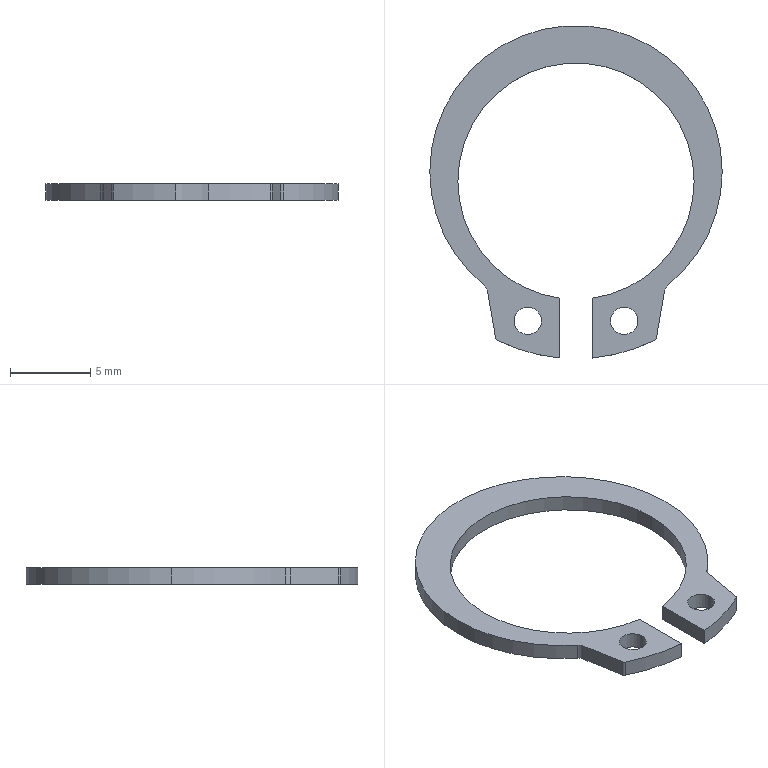Part | SolidWorks | features Extrusion 1 | 1 solid | 22 faces | box 18.2 x 20.685 x 1 mm | volume 106.213 mm3 | cylinder 16 | plane 6 | commonest cylinder face diameters 1.7 x4 14.7 x3 18.2 x3 0.4 x2 1 x2 22.1 x2
STEP:
#1=CARTESIAN_POINT('',(2.15,-9.277,0.5));
#2=VERTEX_POINT('',#1);
#3=CARTESIAN_POINT('',(3.85,-9.277,0.5));
#4=VERTEX_POINT('',#3);
#5=CARTESIAN_POINT('',(3.,-9.277,0.5));
#6=DIRECTION('',(0.,0.,1.));
#7=DIRECTION('',(-1.,0.,0.));
#8=AXIS2_PLACEMENT_3D('',#5,#6,#7);
#9=CIRCLE('',#8,0.85);
#10=EDGE_CURVE('',#2,#4,#9,.T.);
#11=ORIENTED_EDGE('',*,*,#10,.T.);
#12=CARTESIAN_POINT('',(3.85,-9.277,-0.5));
#13=VERTEX_POINT('',#12);
#14=CARTESIAN_POINT('',(3.85,-9.277,0.5));
#15=DIRECTION('',(0.,0.,-1.));
#16=VECTOR('',#15,1000.);
#17=LINE('',#14,#16);
#18=EDGE_CURVE('',#4,#13,#17,.T.);
#19=ORIENTED_EDGE('',*,*,#18,.T.);
#20=CARTESIAN_POINT('',(2.15,-9.277,-0.5));
#21=VERTEX_POINT('',#20);
#22=CARTESIAN_POINT('',(3.,-9.277,-0.5));
#23=DIRECTION('',(0.,0.,1.));
#24=DIRECTION('',(-1.,0.,0.));
#25=AXIS2_PLACEMENT_3D('',#22,#23,#24);
#26=CIRCLE('',#25,0.85);
#27=EDGE_CURVE('',#21,#13,#26,.T.);
#28=ORIENTED_EDGE('',*,*,#27,.F.);
#29=CARTESIAN_POINT('',(2.15,-9.277,0.5));
#30=DIRECTION('',(0.,0.,-1.));
#31=VECTOR('',#30,1000.);
#32=LINE('',#29,#31);
#33=EDGE_CURVE('',#2,#21,#32,.T.);
#34=ORIENTED_EDGE('',*,*,#33,.F.);
#35=EDGE_LOOP('',(#11,#19,#28,#34));
#36=FACE_OUTER_BOUND('',#35,.T.);
#37=CARTESIAN_POINT('',(3.,-9.277,0.5));
#38=DIRECTION('',(0.,0.,-1.));
#39=DIRECTION('',(-1.,0.,0.));
#40=AXIS2_PLACEMENT_3D('',#37,#38,#39);
#41=CYLINDRICAL_SURFACE('',#40,0.85);
#42=ADVANCED_FACE('',(#36),#41,.F.);
#43=CARTESIAN_POINT('',(-3.85,-9.277,0.5));
#44=VERTEX_POINT('',#43);
#45=CARTESIAN_POINT('',(-2.15,-9.277,0.5));
#46=VERTEX_POINT('',#45);
#47=CARTESIAN_POINT('',(-3.,-9.277,0.5));
#48=DIRECTION('',(0.,0.,1.));
#49=DIRECTION('',(1.,0.,0.));
#50=AXIS2_PLACEMENT_3D('',#47,#48,#49);
#51=CIRCLE('',#50,0.85);
#52=EDGE_CURVE('',#44,#46,#51,.T.);
#53=ORIENTED_EDGE('',*,*,#52,.T.);
#54=CARTESIAN_POINT('',(-2.15,-9.277,-0.5));
#55=VERTEX_POINT('',#54);
#56=CARTESIAN_POINT('',(-2.15,-9.277,0.5));
#57=DIRECTION('',(0.,0.,-1.));
#58=VECTOR('',#57,1000.);
#59=LINE('',#56,#58);
#60=EDGE_CURVE('',#46,#55,#59,.T.);
#61=ORIENTED_EDGE('',*,*,#60,.T.);
#62=CARTESIAN_POINT('',(-3.85,-9.277,-0.5));
#63=VERTEX_POINT('',#62);
#64=CARTESIAN_POINT('',(-3.,-9.277,-0.5));
#65=DIRECTION('',(0.,0.,1.));
#66=DIRECTION('',(1.,0.,0.));
#67=AXIS2_PLACEMENT_3D('',#64,#65,#66);
#68=CIRCLE('',#67,0.85);
#69=EDGE_CURVE('',#63,#55,#68,.T.);
#70=ORIENTED_EDGE('',*,*,#69,.F.);
#71=CARTESIAN_POINT('',(-3.85,-9.277,0.5));
#72=DIRECTION('',(0.,0.,-1.));
#73=VECTOR('',#72,1000.);
#74=LINE('',#71,#73);
#75=EDGE_CURVE('',#44,#63,#74,.T.);
#76=ORIENTED_EDGE('',*,*,#75,.F.);
#77=EDGE_LOOP('',(#53,#61,#70,#76));
#78=FACE_OUTER_BOUND('',#77,.T.);
#79=CARTESIAN_POINT('',(-3.,-9.277,0.5));
#80=DIRECTION('',(0.,0.,-1.));
#81=DIRECTION('',(-1.,0.,0.));
#82=AXIS2_PLACEMENT_3D('',#79,#80,#81);
#83=CYLINDRICAL_SURFACE('',#82,0.85);
#84=ADVANCED_FACE('',(#78),#83,.F.);
#85=CARTESIAN_POINT('',(9.1,0.,0.5));
#86=VERTEX_POINT('',#85);
#87=CARTESIAN_POINT('',(-9.1,0.,0.5));
#88=VERTEX_POINT('',#87);
#89=CARTESIAN_POINT('',(0.,0.,0.5));
#90=DIRECTION('',(0.,0.,1.));
#91=DIRECTION('',(1.,0.,0.));
#92=AXIS2_PLACEMENT_3D('',#89,#90,#91);
#93=CIRCLE('',#92,9.1);
#94=EDGE_CURVE('',#86,#88,#93,.T.);
#95=ORIENTED_EDGE('',*,*,#94,.F.);
#96=CARTESIAN_POINT('',(9.1,0.,-0.5));
#97=VERTEX_POINT('',#96);
#98=CARTESIAN_POINT('',(9.1,0.,0.5));
#99=DIRECTION('',(0.,0.,-1.));
#100=VECTOR('',#99,1000.);
#101=LINE('',#98,#100);
#102=EDGE_CURVE('',#86,#97,#101,.T.);
#103=ORIENTED_EDGE('',*,*,#102,.T.);
#104=CARTESIAN_POINT('',(-9.1,0.,-0.5));
#105=VERTEX_POINT('',#104);
#106=CARTESIAN_POINT('',(0.,0.,-0.5));
#107=DIRECTION('',(0.,0.,1.));
#108=DIRECTION('',(1.,0.,0.));
#109=AXIS2_PLACEMENT_3D('',#106,#107,#108);
#110=CIRCLE('',#109,9.1);
#111=EDGE_CURVE('',#97,#105,#110,.T.);
#112=ORIENTED_EDGE('',*,*,#111,.T.);
#113=CARTESIAN_POINT('',(-9.1,0.,0.5));
#114=DIRECTION('',(0.,0.,-1.));
#115=VECTOR('',#114,1000.);
#116=LINE('',#113,#115);
#117=EDGE_CURVE('',#88,#105,#116,.T.);
#118=ORIENTED_EDGE('',*,*,#117,.F.);
#119=EDGE_LOOP('',(#95,#103,#112,#118));
#120=FACE_OUTER_BOUND('',#119,.T.);
#121=CARTESIAN_POINT('',(0.,0.,0.5));
#122=DIRECTION('',(0.,0.,-1.));
#123=DIRECTION('',(-1.,0.,0.));
#124=AXIS2_PLACEMENT_3D('',#121,#122,#123);
#125=CYLINDRICAL_SURFACE('',#124,9.1);
#126=ADVANCED_FACE('',(#120),#125,.T.);
#127=CARTESIAN_POINT('',(-5.699,-7.095,0.5));
#128=VERTEX_POINT('',#127);
#129=CARTESIAN_POINT('',(0.,0.,0.5));
#130=DIRECTION('',(0.,0.,1.));
#131=DIRECTION('',(1.,0.,0.));
#132=AXIS2_PLACEMENT_3D('',#129,#130,#131);
#133=CIRCLE('',#132,9.1);
#134=EDGE_CURVE('',#88,#128,#133,.T.);
#135=ORIENTED_EDGE('',*,*,#134,.F.);
#136=ORIENTED_EDGE('',*,*,#117,.T.);
#137=CARTESIAN_POINT('',(-5.699,-7.095,-0.5));
#138=VERTEX_POINT('',#137);
#139=CARTESIAN_POINT('',(0.,0.,-0.5));
#140=DIRECTION('',(0.,0.,1.));
#141=DIRECTION('',(1.,0.,0.));
#142=AXIS2_PLACEMENT_3D('',#139,#140,#141);
#143=CIRCLE('',#142,9.1);
#144=EDGE_CURVE('',#105,#138,#143,.T.);
#145=ORIENTED_EDGE('',*,*,#144,.T.);
#146=CARTESIAN_POINT('',(-5.699,-7.095,0.5));
#147=DIRECTION('',(0.,0.,-1.));
#148=VECTOR('',#147,1000.);
#149=LINE('',#146,#148);
#150=EDGE_CURVE('',#128,#138,#149,.T.);
#151=ORIENTED_EDGE('',*,*,#150,.F.);
#152=EDGE_LOOP('',(#135,#136,#145,#151));
#153=FACE_OUTER_BOUND('',#152,.T.);
#154=CARTESIAN_POINT('',(0.,0.,0.5));
#155=DIRECTION('',(0.,0.,-1.));
#156=DIRECTION('',(-1.,0.,0.));
#157=AXIS2_PLACEMENT_3D('',#154,#155,#156);
#158=CYLINDRICAL_SURFACE('',#157,9.1);
#159=ADVANCED_FACE('',(#153),#158,.T.);
#160=CARTESIAN_POINT('',(7.35,-0.58,0.5));
#161=VERTEX_POINT('',#160);
#162=CARTESIAN_POINT('',(1.,-7.862,0.5));
#163=VERTEX_POINT('',#162);
#164=CARTESIAN_POINT('',(0.,-0.58,0.5));
#165=DIRECTION('',(0.,0.,-1.));
#166=DIRECTION('',(1.,0.,0.));
#167=AXIS2_PLACEMENT_3D('',#164,#165,#166);
#168=CIRCLE('',#167,7.35);
#169=EDGE_CURVE('',#161,#163,#168,.T.);
#170=ORIENTED_EDGE('',*,*,#169,.F.);
#171=CARTESIAN_POINT('',(7.35,-0.58,-0.5));
#172=VERTEX_POINT('',#171);
#173=CARTESIAN_POINT('',(7.35,-0.58,0.5));
#174=DIRECTION('',(0.,0.,-1.));
#175=VECTOR('',#174,1000.);
#176=LINE('',#173,#175);
#177=EDGE_CURVE('',#161,#172,#176,.T.);
#178=ORIENTED_EDGE('',*,*,#177,.T.);
#179=CARTESIAN_POINT('',(1.,-7.862,-0.5));
#180=VERTEX_POINT('',#179);
#181=CARTESIAN_POINT('',(0.,-0.58,-0.5));
#182=DIRECTION('',(0.,0.,-1.));
#183=DIRECTION('',(1.,0.,0.));
#184=AXIS2_PLACEMENT_3D('',#181,#182,#183);
#185=CIRCLE('',#184,7.35);
#186=EDGE_CURVE('',#172,#180,#185,.T.);
#187=ORIENTED_EDGE('',*,*,#186,.T.);
#188=CARTESIAN_POINT('',(1.,-7.862,0.5));
#189=DIRECTION('',(0.,0.,-1.));
#190=VECTOR('',#189,1000.);
#191=LINE('',#188,#190);
#192=EDGE_CURVE('',#163,#180,#191,.T.);
#193=ORIENTED_EDGE('',*,*,#192,.F.);
#194=EDGE_LOOP('',(#170,#178,#187,#193));
#195=FACE_OUTER_BOUND('',#194,.T.);
#196=CARTESIAN_POINT('',(0.,-0.58,0.5));
#197=DIRECTION('',(0.,0.,-1.));
#198=DIRECTION('',(-1.,0.,0.));
#199=AXIS2_PLACEMENT_3D('',#196,#197,#198);
#200=CYLINDRICAL_SURFACE('',#199,7.35);
#201=ADVANCED_FACE('',(#195),#200,.F.);
#202=ORIENTED_EDGE('',*,*,#177,.F.);
#203=CARTESIAN_POINT('',(-7.35,-0.58,0.5));
#204=VERTEX_POINT('',#203);
#205=CARTESIAN_POINT('',(0.,-0.58,0.5));
#206=DIRECTION('',(0.,0.,-1.));
#207=DIRECTION('',(1.,0.,0.));
#208=AXIS2_PLACEMENT_3D('',#205,#206,#207);
#209=CIRCLE('',#208,7.35);
#210=EDGE_CURVE('',#204,#161,#209,.T.);
#211=ORIENTED_EDGE('',*,*,#210,.F.);
#212=CARTESIAN_POINT('',(-7.35,-0.58,-0.5));
#213=VERTEX_POINT('',#212);
#214=CARTESIAN_POINT('',(-7.35,-0.58,0.5));
#215=DIRECTION('',(0.,0.,-1.));
#216=VECTOR('',#215,1000.);
#217=LINE('',#214,#216);
#218=EDGE_CURVE('',#204,#213,#217,.T.);
#219=ORIENTED_EDGE('',*,*,#218,.T.);
#220=CARTESIAN_POINT('',(0.,-0.58,-0.5));
#221=DIRECTION('',(0.,0.,-1.));
#222=DIRECTION('',(1.,0.,0.));
#223=AXIS2_PLACEMENT_3D('',#220,#221,#222);
#224=CIRCLE('',#223,7.35);
#225=EDGE_CURVE('',#213,#172,#224,.T.);
#226=ORIENTED_EDGE('',*,*,#225,.T.);
#227=EDGE_LOOP('',(#202,#211,#219,#226));
#228=FACE_OUTER_BOUND('',#227,.T.);
#229=CARTESIAN_POINT('',(0.,-0.58,0.5));
#230=DIRECTION('',(0.,0.,-1.));
#231=DIRECTION('',(-1.,0.,0.));
#232=AXIS2_PLACEMENT_3D('',#229,#230,#231);
#233=CYLINDRICAL_SURFACE('',#232,7.35);
#234=ADVANCED_FACE('',(#228),#233,.F.);
#235=ORIENTED_EDGE('',*,*,#52,.F.);
#236=CARTESIAN_POINT('',(-3.,-9.277,0.5));
#237=DIRECTION('',(0.,0.,1.));
#238=DIRECTION('',(1.,0.,0.));
#239=AXIS2_PLACEMENT_3D('',#236,#237,#238);
#240=CIRCLE('',#239,0.85);
#241=EDGE_CURVE('',#46,#44,#240,.T.);
#242=ORIENTED_EDGE('',*,*,#241,.F.);
#243=EDGE_LOOP('',(#235,#242));
#244=FACE_BOUND('',#243,.T.);
#245=CARTESIAN_POINT('',(-5.519,-7.398,0.5));
#246=VERTEX_POINT('',#245);
#247=CARTESIAN_POINT('',(-6.012,-7.484,0.5));
#248=DIRECTION('',(0.,0.,-1.));
#249=DIRECTION('',(1.,0.,0.));
#250=AXIS2_PLACEMENT_3D('',#247,#248,#249);
#251=CIRCLE('',#250,0.5);
#252=EDGE_CURVE('',#128,#246,#251,.T.);
#253=ORIENTED_EDGE('',*,*,#252,.T.);
#254=CARTESIAN_POINT('',(-5.,-10.344,0.5));
#255=VERTEX_POINT('',#254);
#256=CARTESIAN_POINT('',(-5.519,-7.398,0.5));
#257=DIRECTION('',(0.1736,-0.9848,0.));
#258=VECTOR('',#257,1000.);
#259=LINE('',#256,#258);
#260=EDGE_CURVE('',#246,#255,#259,.T.);
#261=ORIENTED_EDGE('',*,*,#260,.T.);
#262=CARTESIAN_POINT('',(-4.892,-10.488,0.5));
#263=VERTEX_POINT('',#262);
#264=CARTESIAN_POINT('',(-4.803,-10.309,0.5));
#265=DIRECTION('',(0.,0.,1.));
#266=DIRECTION('',(-1.,0.,0.));
#267=AXIS2_PLACEMENT_3D('',#264,#265,#266);
#268=CIRCLE('',#267,0.2);
#269=EDGE_CURVE('',#255,#263,#268,.T.);
#270=ORIENTED_EDGE('',*,*,#269,.T.);
#271=CARTESIAN_POINT('',(-1.,-11.585,0.5));
#272=VERTEX_POINT('',#271);
#273=CARTESIAN_POINT('',(0.,-0.58,0.5));
#274=DIRECTION('',(0.,0.,1.));
#275=DIRECTION('',(-1.,0.,0.));
#276=AXIS2_PLACEMENT_3D('',#273,#274,#275);
#277=CIRCLE('',#276,11.05);
#278=EDGE_CURVE('',#263,#272,#277,.T.);
#279=ORIENTED_EDGE('',*,*,#278,.T.);
#280=CARTESIAN_POINT('',(-1.,-7.862,0.5));
#281=VERTEX_POINT('',#280);
#282=CARTESIAN_POINT('',(-1.,-7.862,0.5));
#283=DIRECTION('',(0.,1.,0.));
#284=VECTOR('',#283,1000.);
#285=LINE('',#282,#284);
#286=EDGE_CURVE('',#272,#281,#285,.T.);
#287=ORIENTED_EDGE('',*,*,#286,.T.);
#288=CARTESIAN_POINT('',(0.,-0.58,0.5));
#289=DIRECTION('',(0.,0.,-1.));
#290=DIRECTION('',(1.,0.,0.));
#291=AXIS2_PLACEMENT_3D('',#288,#289,#290);
#292=CIRCLE('',#291,7.35);
#293=EDGE_CURVE('',#281,#204,#292,.T.);
#294=ORIENTED_EDGE('',*,*,#293,.T.);
#295=ORIENTED_EDGE('',*,*,#210,.T.);
#296=ORIENTED_EDGE('',*,*,#169,.T.);
#297=CARTESIAN_POINT('',(1.,-11.585,0.5));
#298=VERTEX_POINT('',#297);
#299=CARTESIAN_POINT('',(1.,-7.862,0.5));
#300=DIRECTION('',(0.,-1.,0.));
#301=VECTOR('',#300,1000.);
#302=LINE('',#299,#301);
#303=EDGE_CURVE('',#163,#298,#302,.T.);
#304=ORIENTED_EDGE('',*,*,#303,.T.);
#305=CARTESIAN_POINT('',(4.892,-10.488,0.5));
#306=VERTEX_POINT('',#305);
#307=CARTESIAN_POINT('',(0.,-0.58,0.5));
#308=DIRECTION('',(0.,0.,1.));
#309=DIRECTION('',(1.,0.,0.));
#310=AXIS2_PLACEMENT_3D('',#307,#308,#309);
#311=CIRCLE('',#310,11.05);
#312=EDGE_CURVE('',#298,#306,#311,.T.);
#313=ORIENTED_EDGE('',*,*,#312,.T.);
#314=CARTESIAN_POINT('',(5.,-10.344,0.5));
#315=VERTEX_POINT('',#314);
#316=CARTESIAN_POINT('',(4.803,-10.309,0.5));
#317=DIRECTION('',(0.,0.,1.));
#318=DIRECTION('',(1.,0.,0.));
#319=AXIS2_PLACEMENT_3D('',#316,#317,#318);
#320=CIRCLE('',#319,0.2);
#321=EDGE_CURVE('',#306,#315,#320,.T.);
#322=ORIENTED_EDGE('',*,*,#321,.T.);
#323=CARTESIAN_POINT('',(5.519,-7.398,0.5));
#324=VERTEX_POINT('',#323);
#325=CARTESIAN_POINT('',(5.519,-7.398,0.5));
#326=DIRECTION('',(0.1736,0.9848,0.));
#327=VECTOR('',#326,1000.);
#328=LINE('',#325,#327);
#329=EDGE_CURVE('',#315,#324,#328,.T.);
#330=ORIENTED_EDGE('',*,*,#329,.T.);
#331=CARTESIAN_POINT('',(5.699,-7.095,0.5));
#332=VERTEX_POINT('',#331);
#333=CARTESIAN_POINT('',(6.012,-7.484,0.5));
#334=DIRECTION('',(0.,0.,-1.));
#335=DIRECTION('',(-1.,0.,0.));
#336=AXIS2_PLACEMENT_3D('',#333,#334,#335);
#337=CIRCLE('',#336,0.5);
#338=EDGE_CURVE('',#324,#332,#337,.T.);
#339=ORIENTED_EDGE('',*,*,#338,.T.);
#340=CARTESIAN_POINT('',(0.,0.,0.5));
#341=DIRECTION('',(0.,0.,1.));
#342=DIRECTION('',(1.,0.,0.));
#343=AXIS2_PLACEMENT_3D('',#340,#341,#342);
#344=CIRCLE('',#343,9.1);
#345=EDGE_CURVE('',#332,#86,#344,.T.);
#346=ORIENTED_EDGE('',*,*,#345,.T.);
#347=ORIENTED_EDGE('',*,*,#94,.T.);
#348=ORIENTED_EDGE('',*,*,#134,.T.);
#349=EDGE_LOOP('',(#253,#261,#270,#279,#287,#294,#295,#296,#304,#313,#322,#330,#339,#346,#347,#348));
#350=FACE_OUTER_BOUND('',#349,.T.);
#351=ORIENTED_EDGE('',*,*,#10,.F.);
#352=CARTESIAN_POINT('',(3.,-9.277,0.5));
#353=DIRECTION('',(0.,0.,1.));
#354=DIRECTION('',(-1.,0.,0.));
#355=AXIS2_PLACEMENT_3D('',#352,#353,#354);
#356=CIRCLE('',#355,0.85);
#357=EDGE_CURVE('',#4,#2,#356,.T.);
#358=ORIENTED_EDGE('',*,*,#357,.F.);
#359=EDGE_LOOP('',(#351,#358));
#360=FACE_BOUND('',#359,.T.);
#361=CARTESIAN_POINT('',(-6.012,-7.484,0.5));
#362=DIRECTION('',(0.,0.,1.));
#363=DIRECTION('',(1.,0.,0.));
#364=AXIS2_PLACEMENT_3D('',#361,#362,#363);
#365=PLANE('',#364);
#366=ADVANCED_FACE('',(#244,#350,#360),#365,.T.);
#367=ORIENTED_EDGE('',*,*,#150,.T.);
#368=CARTESIAN_POINT('',(-5.519,-7.398,-0.5));
#369=VERTEX_POINT('',#368);
#370=CARTESIAN_POINT('',(-6.012,-7.484,-0.5));
#371=DIRECTION('',(0.,0.,-1.));
#372=DIRECTION('',(1.,0.,0.));
#373=AXIS2_PLACEMENT_3D('',#370,#371,#372);
#374=CIRCLE('',#373,0.5);
#375=EDGE_CURVE('',#138,#369,#374,.T.);
#376=ORIENTED_EDGE('',*,*,#375,.T.);
#377=CARTESIAN_POINT('',(-5.519,-7.398,0.5));
#378=DIRECTION('',(0.,0.,-1.));
#379=VECTOR('',#378,1000.);
#380=LINE('',#377,#379);
#381=EDGE_CURVE('',#246,#369,#380,.T.);
#382=ORIENTED_EDGE('',*,*,#381,.F.);
#383=ORIENTED_EDGE('',*,*,#252,.F.);
#384=EDGE_LOOP('',(#367,#376,#382,#383));
#385=FACE_OUTER_BOUND('',#384,.T.);
#386=CARTESIAN_POINT('',(-6.012,-7.484,0.5));
#387=DIRECTION('',(0.,0.,-1.));
#388=DIRECTION('',(-1.,0.,0.));
#389=AXIS2_PLACEMENT_3D('',#386,#387,#388);
#390=CYLINDRICAL_SURFACE('',#389,0.5);
#391=ADVANCED_FACE('',(#385),#390,.F.);
#392=ORIENTED_EDGE('',*,*,#381,.T.);
#393=CARTESIAN_POINT('',(-5.,-10.344,-0.5));
#394=VERTEX_POINT('',#393);
#395=CARTESIAN_POINT('',(-5.519,-7.398,-0.5));
#396=DIRECTION('',(0.1736,-0.9848,0.));
#397=VECTOR('',#396,1000.);
#398=LINE('',#395,#397);
#399=EDGE_CURVE('',#369,#394,#398,.T.);
#400=ORIENTED_EDGE('',*,*,#399,.T.);
#401=CARTESIAN_POINT('',(-5.,-10.344,0.5));
#402=DIRECTION('',(0.,0.,-1.));
#403=VECTOR('',#402,1000.);
#404=LINE('',#401,#403);
#405=EDGE_CURVE('',#255,#394,#404,.T.);
#406=ORIENTED_EDGE('',*,*,#405,.F.);
#407=ORIENTED_EDGE('',*,*,#260,.F.);
#408=EDGE_LOOP('',(#392,#400,#406,#407));
#409=FACE_OUTER_BOUND('',#408,.T.);
#410=CARTESIAN_POINT('',(-5.519,-7.398,0.5));
#411=DIRECTION('',(0.9848,0.1736,0.));
#412=DIRECTION('',(-0.1736,0.9848,0.));
#413=AXIS2_PLACEMENT_3D('',#410,#411,#412);
#414=PLANE('',#413);
#415=ADVANCED_FACE('',(#409),#414,.F.);
#416=ORIENTED_EDGE('',*,*,#405,.T.);
#417=CARTESIAN_POINT('',(-4.892,-10.488,-0.5));
#418=VERTEX_POINT('',#417);
#419=CARTESIAN_POINT('',(-4.803,-10.309,-0.5));
#420=DIRECTION('',(0.,0.,1.));
#421=DIRECTION('',(-1.,0.,0.));
#422=AXIS2_PLACEMENT_3D('',#419,#420,#421);
#423=CIRCLE('',#422,0.2);
#424=EDGE_CURVE('',#394,#418,#423,.T.);
#425=ORIENTED_EDGE('',*,*,#424,.T.);
#426=CARTESIAN_POINT('',(-4.892,-10.488,0.5));
#427=DIRECTION('',(0.,0.,-1.));
#428=VECTOR('',#427,1000.);
#429=LINE('',#426,#428);
#430=EDGE_CURVE('',#263,#418,#429,.T.);
#431=ORIENTED_EDGE('',*,*,#430,.F.);
#432=ORIENTED_EDGE('',*,*,#269,.F.);
#433=EDGE_LOOP('',(#416,#425,#431,#432));
#434=FACE_OUTER_BOUND('',#433,.T.);
#435=CARTESIAN_POINT('',(-4.803,-10.309,0.5));
#436=DIRECTION('',(0.,0.,-1.));
#437=DIRECTION('',(-1.,0.,0.));
#438=AXIS2_PLACEMENT_3D('',#435,#436,#437);
#439=CYLINDRICAL_SURFACE('',#438,0.2);
#440=ADVANCED_FACE('',(#434),#439,.T.);
#441=ORIENTED_EDGE('',*,*,#430,.T.);
#442=CARTESIAN_POINT('',(-1.,-11.585,-0.5));
#443=VERTEX_POINT('',#442);
#444=CARTESIAN_POINT('',(0.,-0.58,-0.5));
#445=DIRECTION('',(0.,0.,1.));
#446=DIRECTION('',(-1.,0.,0.));
#447=AXIS2_PLACEMENT_3D('',#444,#445,#446);
#448=CIRCLE('',#447,11.05);
#449=EDGE_CURVE('',#418,#443,#448,.T.);
#450=ORIENTED_EDGE('',*,*,#449,.T.);
#451=CARTESIAN_POINT('',(-1.,-11.585,0.5));
#452=DIRECTION('',(0.,0.,-1.));
#453=VECTOR('',#452,1000.);
#454=LINE('',#451,#453);
#455=EDGE_CURVE('',#272,#443,#454,.T.);
#456=ORIENTED_EDGE('',*,*,#455,.F.);
#457=ORIENTED_EDGE('',*,*,#278,.F.);
#458=EDGE_LOOP('',(#441,#450,#456,#457));
#459=FACE_OUTER_BOUND('',#458,.T.);
#460=CARTESIAN_POINT('',(0.,-0.58,0.5));
#461=DIRECTION('',(0.,0.,-1.));
#462=DIRECTION('',(-1.,0.,0.));
#463=AXIS2_PLACEMENT_3D('',#460,#461,#462);
#464=CYLINDRICAL_SURFACE('',#463,11.05);
#465=ADVANCED_FACE('',(#459),#464,.T.);
#466=ORIENTED_EDGE('',*,*,#455,.T.);
#467=CARTESIAN_POINT('',(-1.,-7.862,-0.5));
#468=VERTEX_POINT('',#467);
#469=CARTESIAN_POINT('',(-1.,-7.862,-0.5));
#470=DIRECTION('',(0.,1.,0.));
#471=VECTOR('',#470,1000.);
#472=LINE('',#469,#471);
#473=EDGE_CURVE('',#443,#468,#472,.T.);
#474=ORIENTED_EDGE('',*,*,#473,.T.);
#475=CARTESIAN_POINT('',(-1.,-7.862,0.5));
#476=DIRECTION('',(0.,0.,-1.));
#477=VECTOR('',#476,1000.);
#478=LINE('',#475,#477);
#479=EDGE_CURVE('',#281,#468,#478,.T.);
#480=ORIENTED_EDGE('',*,*,#479,.F.);
#481=ORIENTED_EDGE('',*,*,#286,.F.);
#482=EDGE_LOOP('',(#466,#474,#480,#481));
#483=FACE_OUTER_BOUND('',#482,.T.);
#484=CARTESIAN_POINT('',(-1.,-7.862,0.5));
#485=DIRECTION('',(-1.,0.,0.));
#486=DIRECTION('',(0.,-1.,0.));
#487=AXIS2_PLACEMENT_3D('',#484,#485,#486);
#488=PLANE('',#487);
#489=ADVANCED_FACE('',(#483),#488,.F.);
#490=ORIENTED_EDGE('',*,*,#218,.F.);
#491=ORIENTED_EDGE('',*,*,#293,.F.);
#492=ORIENTED_EDGE('',*,*,#479,.T.);
#493=CARTESIAN_POINT('',(0.,-0.58,-0.5));
#494=DIRECTION('',(0.,0.,-1.));
#495=DIRECTION('',(1.,0.,0.));
#496=AXIS2_PLACEMENT_3D('',#493,#494,#495);
#497=CIRCLE('',#496,7.35);
#498=EDGE_CURVE('',#468,#213,#497,.T.);
#499=ORIENTED_EDGE('',*,*,#498,.T.);
#500=EDGE_LOOP('',(#490,#491,#492,#499));
#501=FACE_OUTER_BOUND('',#500,.T.);
#502=CARTESIAN_POINT('',(0.,-0.58,0.5));
#503=DIRECTION('',(0.,0.,-1.));
#504=DIRECTION('',(-1.,0.,0.));
#505=AXIS2_PLACEMENT_3D('',#502,#503,#504);
#506=CYLINDRICAL_SURFACE('',#505,7.35);
#507=ADVANCED_FACE('',(#501),#506,.F.);
#508=ORIENTED_EDGE('',*,*,#192,.T.);
#509=CARTESIAN_POINT('',(1.,-11.585,-0.5));
#510=VERTEX_POINT('',#509);
#511=CARTESIAN_POINT('',(1.,-7.862,-0.5));
#512=DIRECTION('',(0.,-1.,0.));
#513=VECTOR('',#512,1000.);
#514=LINE('',#511,#513);
#515=EDGE_CURVE('',#180,#510,#514,.T.);
#516=ORIENTED_EDGE('',*,*,#515,.T.);
#517=CARTESIAN_POINT('',(1.,-11.585,0.5));
#518=DIRECTION('',(0.,0.,-1.));
#519=VECTOR('',#518,1000.);
#520=LINE('',#517,#519);
#521=EDGE_CURVE('',#298,#510,#520,.T.);
#522=ORIENTED_EDGE('',*,*,#521,.F.);
#523=ORIENTED_EDGE('',*,*,#303,.F.);
#524=EDGE_LOOP('',(#508,#516,#522,#523));
#525=FACE_OUTER_BOUND('',#524,.T.);
#526=CARTESIAN_POINT('',(1.,-7.862,0.5));
#527=DIRECTION('',(1.,0.,0.));
#528=DIRECTION('',(0.,0.,-1.));
#529=AXIS2_PLACEMENT_3D('',#526,#527,#528);
#530=PLANE('',#529);
#531=ADVANCED_FACE('',(#525),#530,.F.);
#532=ORIENTED_EDGE('',*,*,#521,.T.);
#533=CARTESIAN_POINT('',(4.892,-10.488,-0.5));
#534=VERTEX_POINT('',#533);
#535=CARTESIAN_POINT('',(0.,-0.58,-0.5));
#536=DIRECTION('',(0.,0.,1.));
#537=DIRECTION('',(1.,0.,0.));
#538=AXIS2_PLACEMENT_3D('',#535,#536,#537);
#539=CIRCLE('',#538,11.05);
#540=EDGE_CURVE('',#510,#534,#539,.T.);
#541=ORIENTED_EDGE('',*,*,#540,.T.);
#542=CARTESIAN_POINT('',(4.892,-10.488,0.5));
#543=DIRECTION('',(0.,0.,-1.));
#544=VECTOR('',#543,1000.);
#545=LINE('',#542,#544);
#546=EDGE_CURVE('',#306,#534,#545,.T.);
#547=ORIENTED_EDGE('',*,*,#546,.F.);
#548=ORIENTED_EDGE('',*,*,#312,.F.);
#549=EDGE_LOOP('',(#532,#541,#547,#548));
#550=FACE_OUTER_BOUND('',#549,.T.);
#551=CARTESIAN_POINT('',(0.,-0.58,0.5));
#552=DIRECTION('',(0.,0.,-1.));
#553=DIRECTION('',(-1.,0.,0.));
#554=AXIS2_PLACEMENT_3D('',#551,#552,#553);
#555=CYLINDRICAL_SURFACE('',#554,11.05);
#556=ADVANCED_FACE('',(#550),#555,.T.);
#557=ORIENTED_EDGE('',*,*,#546,.T.);
#558=CARTESIAN_POINT('',(5.,-10.344,-0.5));
#559=VERTEX_POINT('',#558);
#560=CARTESIAN_POINT('',(4.803,-10.309,-0.5));
#561=DIRECTION('',(0.,0.,1.));
#562=DIRECTION('',(1.,0.,0.));
#563=AXIS2_PLACEMENT_3D('',#560,#561,#562);
#564=CIRCLE('',#563,0.2);
#565=EDGE_CURVE('',#534,#559,#564,.T.);
#566=ORIENTED_EDGE('',*,*,#565,.T.);
#567=CARTESIAN_POINT('',(5.,-10.344,0.5));
#568=DIRECTION('',(0.,0.,-1.));
#569=VECTOR('',#568,1000.);
#570=LINE('',#567,#569);
#571=EDGE_CURVE('',#315,#559,#570,.T.);
#572=ORIENTED_EDGE('',*,*,#571,.F.);
#573=ORIENTED_EDGE('',*,*,#321,.F.);
#574=EDGE_LOOP('',(#557,#566,#572,#573));
#575=FACE_OUTER_BOUND('',#574,.T.);
#576=CARTESIAN_POINT('',(4.803,-10.309,0.5));
#577=DIRECTION('',(0.,0.,-1.));
#578=DIRECTION('',(-1.,0.,0.));
#579=AXIS2_PLACEMENT_3D('',#576,#577,#578);
#580=CYLINDRICAL_SURFACE('',#579,0.2);
#581=ADVANCED_FACE('',(#575),#580,.T.);
#582=ORIENTED_EDGE('',*,*,#571,.T.);
#583=CARTESIAN_POINT('',(5.519,-7.398,-0.5));
#584=VERTEX_POINT('',#583);
#585=CARTESIAN_POINT('',(5.519,-7.398,-0.5));
#586=DIRECTION('',(0.1736,0.9848,0.));
#587=VECTOR('',#586,1000.);
#588=LINE('',#585,#587);
#589=EDGE_CURVE('',#559,#584,#588,.T.);
#590=ORIENTED_EDGE('',*,*,#589,.T.);
#591=CARTESIAN_POINT('',(5.519,-7.398,0.5));
#592=DIRECTION('',(0.,0.,-1.));
#593=VECTOR('',#592,1000.);
#594=LINE('',#591,#593);
#595=EDGE_CURVE('',#324,#584,#594,.T.);
#596=ORIENTED_EDGE('',*,*,#595,.F.);
#597=ORIENTED_EDGE('',*,*,#329,.F.);
#598=EDGE_LOOP('',(#582,#590,#596,#597));
#599=FACE_OUTER_BOUND('',#598,.T.);
#600=CARTESIAN_POINT('',(5.519,-7.398,0.5));
#601=DIRECTION('',(-0.9848,0.1736,0.));
#602=DIRECTION('',(-0.1736,-0.9848,0.));
#603=AXIS2_PLACEMENT_3D('',#600,#601,#602);
#604=PLANE('',#603);
#605=ADVANCED_FACE('',(#599),#604,.F.);
#606=ORIENTED_EDGE('',*,*,#595,.T.);
#607=CARTESIAN_POINT('',(5.699,-7.095,-0.5));
#608=VERTEX_POINT('',#607);
#609=CARTESIAN_POINT('',(6.012,-7.484,-0.5));
#610=DIRECTION('',(0.,0.,-1.));
#611=DIRECTION('',(-1.,0.,0.));
#612=AXIS2_PLACEMENT_3D('',#609,#610,#611);
#613=CIRCLE('',#612,0.5);
#614=EDGE_CURVE('',#584,#608,#613,.T.);
#615=ORIENTED_EDGE('',*,*,#614,.T.);
#616=CARTESIAN_POINT('',(5.699,-7.095,0.5));
#617=DIRECTION('',(0.,0.,-1.));
#618=VECTOR('',#617,1000.);
#619=LINE('',#616,#618);
#620=EDGE_CURVE('',#332,#608,#619,.T.);
#621=ORIENTED_EDGE('',*,*,#620,.F.);
#622=ORIENTED_EDGE('',*,*,#338,.F.);
#623=EDGE_LOOP('',(#606,#615,#621,#622));
#624=FACE_OUTER_BOUND('',#623,.T.);
#625=CARTESIAN_POINT('',(6.012,-7.484,0.5));
#626=DIRECTION('',(0.,0.,-1.));
#627=DIRECTION('',(-1.,0.,0.));
#628=AXIS2_PLACEMENT_3D('',#625,#626,#627);
#629=CYLINDRICAL_SURFACE('',#628,0.5);
#630=ADVANCED_FACE('',(#624),#629,.F.);
#631=ORIENTED_EDGE('',*,*,#102,.F.);
#632=ORIENTED_EDGE('',*,*,#345,.F.);
#633=ORIENTED_EDGE('',*,*,#620,.T.);
#634=CARTESIAN_POINT('',(0.,0.,-0.5));
#635=DIRECTION('',(0.,0.,1.));
#636=DIRECTION('',(1.,0.,0.));
#637=AXIS2_PLACEMENT_3D('',#634,#635,#636);
#638=CIRCLE('',#637,9.1);
#639=EDGE_CURVE('',#608,#97,#638,.T.);
#640=ORIENTED_EDGE('',*,*,#639,.T.);
#641=EDGE_LOOP('',(#631,#632,#633,#640));
#642=FACE_OUTER_BOUND('',#641,.T.);
#643=CARTESIAN_POINT('',(0.,0.,0.5));
#644=DIRECTION('',(0.,0.,-1.));
#645=DIRECTION('',(-1.,0.,0.));
#646=AXIS2_PLACEMENT_3D('',#643,#644,#645);
#647=CYLINDRICAL_SURFACE('',#646,9.1);
#648=ADVANCED_FACE('',(#642),#647,.T.);
#649=ORIENTED_EDGE('',*,*,#60,.F.);
#650=ORIENTED_EDGE('',*,*,#241,.T.);
#651=ORIENTED_EDGE('',*,*,#75,.T.);
#652=CARTESIAN_POINT('',(-3.,-9.277,-0.5));
#653=DIRECTION('',(0.,0.,1.));
#654=DIRECTION('',(1.,0.,0.));
#655=AXIS2_PLACEMENT_3D('',#652,#653,#654);
#656=CIRCLE('',#655,0.85);
#657=EDGE_CURVE('',#55,#63,#656,.T.);
#658=ORIENTED_EDGE('',*,*,#657,.F.);
#659=EDGE_LOOP('',(#649,#650,#651,#658));
#660=FACE_OUTER_BOUND('',#659,.T.);
#661=CARTESIAN_POINT('',(-3.,-9.277,0.5));
#662=DIRECTION('',(0.,0.,-1.));
#663=DIRECTION('',(-1.,0.,0.));
#664=AXIS2_PLACEMENT_3D('',#661,#662,#663);
#665=CYLINDRICAL_SURFACE('',#664,0.85);
#666=ADVANCED_FACE('',(#660),#665,.F.);
#667=ORIENTED_EDGE('',*,*,#18,.F.);
#668=ORIENTED_EDGE('',*,*,#357,.T.);
#669=ORIENTED_EDGE('',*,*,#33,.T.);
#670=CARTESIAN_POINT('',(3.,-9.277,-0.5));
#671=DIRECTION('',(0.,0.,1.));
#672=DIRECTION('',(-1.,0.,0.));
#673=AXIS2_PLACEMENT_3D('',#670,#671,#672);
#674=CIRCLE('',#673,0.85);
#675=EDGE_CURVE('',#13,#21,#674,.T.);
#676=ORIENTED_EDGE('',*,*,#675,.F.);
#677=EDGE_LOOP('',(#667,#668,#669,#676));
#678=FACE_OUTER_BOUND('',#677,.T.);
#679=CARTESIAN_POINT('',(3.,-9.277,0.5));
#680=DIRECTION('',(0.,0.,-1.));
#681=DIRECTION('',(-1.,0.,0.));
#682=AXIS2_PLACEMENT_3D('',#679,#680,#681);
#683=CYLINDRICAL_SURFACE('',#682,0.85);
#684=ADVANCED_FACE('',(#678),#683,.F.);
#685=ORIENTED_EDGE('',*,*,#27,.T.);
#686=ORIENTED_EDGE('',*,*,#675,.T.);
#687=EDGE_LOOP('',(#685,#686));
#688=FACE_BOUND('',#687,.T.);
#689=ORIENTED_EDGE('',*,*,#69,.T.);
#690=ORIENTED_EDGE('',*,*,#657,.T.);
#691=EDGE_LOOP('',(#689,#690));
#692=FACE_BOUND('',#691,.T.);
#693=ORIENTED_EDGE('',*,*,#375,.F.);
#694=ORIENTED_EDGE('',*,*,#144,.F.);
#695=ORIENTED_EDGE('',*,*,#111,.F.);
#696=ORIENTED_EDGE('',*,*,#639,.F.);
#697=ORIENTED_EDGE('',*,*,#614,.F.);
#698=ORIENTED_EDGE('',*,*,#589,.F.);
#699=ORIENTED_EDGE('',*,*,#565,.F.);
#700=ORIENTED_EDGE('',*,*,#540,.F.);
#701=ORIENTED_EDGE('',*,*,#515,.F.);
#702=ORIENTED_EDGE('',*,*,#186,.F.);
#703=ORIENTED_EDGE('',*,*,#225,.F.);
#704=ORIENTED_EDGE('',*,*,#498,.F.);
#705=ORIENTED_EDGE('',*,*,#473,.F.);
#706=ORIENTED_EDGE('',*,*,#449,.F.);
#707=ORIENTED_EDGE('',*,*,#424,.F.);
#708=ORIENTED_EDGE('',*,*,#399,.F.);
#709=EDGE_LOOP('',(#693,#694,#695,#696,#697,#698,#699,#700,#701,#702,#703,#704,#705,#706,#707,#708));
#710=FACE_OUTER_BOUND('',#709,.T.);
#711=CARTESIAN_POINT('',(-6.012,-7.484,-0.5));
#712=DIRECTION('',(0.,0.,1.));
#713=DIRECTION('',(1.,0.,0.));
#714=AXIS2_PLACEMENT_3D('',#711,#712,#713);
#715=PLANE('',#714);
#716=ADVANCED_FACE('',(#688,#692,#710),#715,.F.);
#717=CLOSED_SHELL('',(#42,#84,#126,#159,#201,#234,#366,#391,#415,#440,#465,#489,#507,#531,#556,#581,#605,#630,#648,#666,#684,#716));
#718=MANIFOLD_SOLID_BREP('',#717);
#719=CARTESIAN_POINT('',(0.,0.,0.));
#720=DIRECTION('',(0.,0.,1.));
#721=DIRECTION('',(1.,0.,0.));
#722=AXIS2_PLACEMENT_3D('',#719,#720,#721);
#723=(LENGTH_UNIT()NAMED_UNIT(*)SI_UNIT(.MILLI.,.METRE.));
#724=UNCERTAINTY_MEASURE_WITH_UNIT(LENGTH_MEASURE(0.00001),#723,'','');
#725=(NAMED_UNIT(*)PLANE_ANGLE_UNIT()SI_UNIT($,.RADIAN.));
#726=(NAMED_UNIT(*)SI_UNIT($,.STERADIAN.)SOLID_ANGLE_UNIT());
#727=(GEOMETRIC_REPRESENTATION_CONTEXT(3)GLOBAL_UNCERTAINTY_ASSIGNED_CONTEXT((#724))GLOBAL_UNIT_ASSIGNED_CONTEXT((#723,#725,#726))REPRESENTATION_CONTEXT('',''));
#728=ADVANCED_BREP_SHAPE_REPRESENTATION('',(#718,#722),#727);